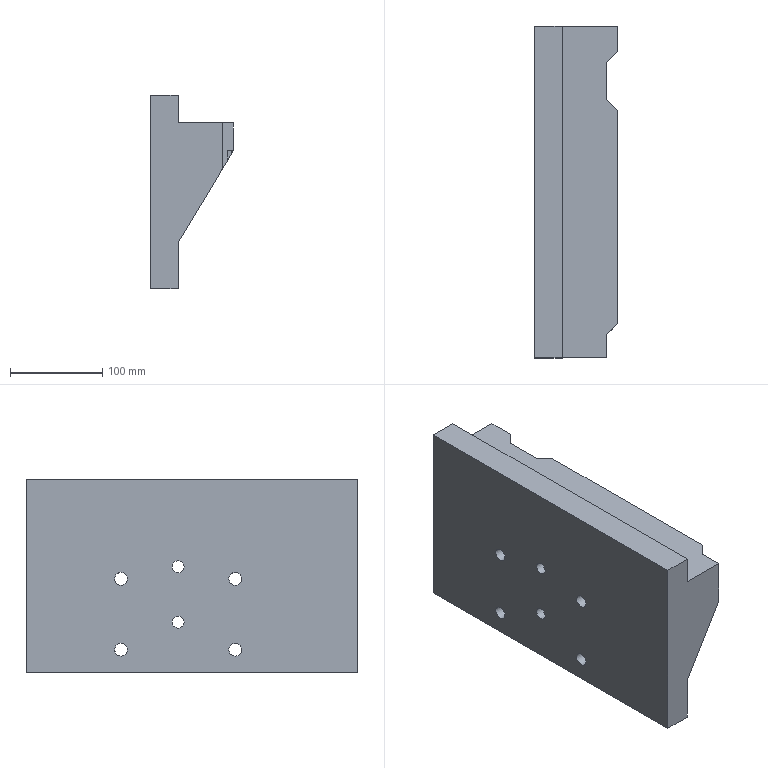Part | NX | features solid 2 | 1 solid | 34 faces | box 90 x 360 x 210 mm | volume 3029888 mm3 | plane 24 | cylinder 10 | commonest cylinder face diameters 14 x4 20 x4 13 x2
STEP:
#1=CARTESIAN_POINT('',(-737.,-445.,40.));
#2=VERTEX_POINT('',#1);
#3=CARTESIAN_POINT('',(-737.,-445.,-10.));
#4=VERTEX_POINT('',#3);
#5=CARTESIAN_POINT('',(-737.,-445.,14.964));
#6=DIRECTION('',(0.,0.,1.));
#7=VECTOR('',#6,1000.);
#8=LINE('',#5,#7);
#9=EDGE_CURVE('',#2,#4,#8,.F.);
#10=ORIENTED_EDGE('',*,*,#9,.F.);
#11=CARTESIAN_POINT('',(-785.,-445.,40.));
#12=VERTEX_POINT('',#11);
#13=CARTESIAN_POINT('',(-785.,-445.,40.));
#14=DIRECTION('',(1.,0.,0.));
#15=VECTOR('',#14,1000.);
#16=LINE('',#13,#15);
#17=EDGE_CURVE('',#12,#2,#16,.T.);
#18=ORIENTED_EDGE('',*,*,#17,.F.);
#19=CARTESIAN_POINT('',(-785.,-445.,70.));
#20=VERTEX_POINT('',#19);
#21=CARTESIAN_POINT('',(-785.,-445.,69.026));
#22=DIRECTION('',(0.,0.,1.));
#23=VECTOR('',#22,1000.);
#24=LINE('',#21,#23);
#25=EDGE_CURVE('',#20,#12,#24,.F.);
#26=ORIENTED_EDGE('',*,*,#25,.F.);
#27=CARTESIAN_POINT('',(-815.,-445.,70.));
#28=VERTEX_POINT('',#27);
#29=CARTESIAN_POINT('',(-785.,-445.,70.));
#30=DIRECTION('',(-1.,0.,0.));
#31=VECTOR('',#30,1000.);
#32=LINE('',#29,#31);
#33=EDGE_CURVE('',#20,#28,#32,.T.);
#34=ORIENTED_EDGE('',*,*,#33,.T.);
#35=CARTESIAN_POINT('',(-815.,-445.,-140.));
#36=VERTEX_POINT('',#35);
#37=CARTESIAN_POINT('',(-815.,-445.,69.026));
#38=DIRECTION('',(0.,0.,1.));
#39=VECTOR('',#38,1000.);
#40=LINE('',#37,#39);
#41=EDGE_CURVE('',#28,#36,#40,.F.);
#42=ORIENTED_EDGE('',*,*,#41,.T.);
#43=CARTESIAN_POINT('',(-785.,-445.,-140.));
#44=VERTEX_POINT('',#43);
#45=CARTESIAN_POINT('',(-815.,-445.,-140.));
#46=DIRECTION('',(-1.,0.,0.));
#47=VECTOR('',#46,1000.);
#48=LINE('',#45,#47);
#49=EDGE_CURVE('',#44,#36,#48,.T.);
#50=ORIENTED_EDGE('',*,*,#49,.F.);
#51=CARTESIAN_POINT('',(-785.,-445.,-90.));
#52=VERTEX_POINT('',#51);
#53=CARTESIAN_POINT('',(-785.,-445.,0.));
#54=DIRECTION('',(0.,0.,1.));
#55=VECTOR('',#54,1000.);
#56=LINE('',#53,#55);
#57=EDGE_CURVE('',#52,#44,#56,.F.);
#58=ORIENTED_EDGE('',*,*,#57,.F.);
#59=CARTESIAN_POINT('',(-740.882,-445.,-16.471));
#60=DIRECTION('',(-0.5145,0.,-0.8575));
#61=VECTOR('',#60,1000.);
#62=LINE('',#59,#61);
#63=EDGE_CURVE('',#4,#52,#62,.T.);
#64=ORIENTED_EDGE('',*,*,#63,.F.);
#65=EDGE_LOOP('',(#10,#18,#26,#34,#42,#50,#58,#64));
#66=FACE_BOUND('',#65,.T.);
#67=CARTESIAN_POINT('',(-785.,-445.,14.964));
#68=DIRECTION('',(0.,-1.,0.));
#69=DIRECTION('',(0.,0.,-1.));
#70=AXIS2_PLACEMENT_3D('',#67,#68,#69);
#71=PLANE('',#70);
#72=ADVANCED_FACE('',(#66),#71,.T.);
#73=CARTESIAN_POINT('',(-725.,-113.,40.));
#74=VERTEX_POINT('',#73);
#75=CARTESIAN_POINT('',(-725.,-85.,40.));
#76=VERTEX_POINT('',#75);
#77=CARTESIAN_POINT('',(-725.,-415.,40.));
#78=DIRECTION('',(0.,-1.,0.));
#79=VECTOR('',#78,1000.);
#80=LINE('',#77,#79);
#81=EDGE_CURVE('',#74,#76,#80,.F.);
#82=ORIENTED_EDGE('',*,*,#81,.F.);
#83=CARTESIAN_POINT('',(-725.,-113.,10.));
#84=VERTEX_POINT('',#83);
#85=CARTESIAN_POINT('',(-725.,-113.,60.));
#86=DIRECTION('',(0.,0.,-1.));
#87=VECTOR('',#86,1000.);
#88=LINE('',#85,#87);
#89=EDGE_CURVE('',#74,#84,#88,.T.);
#90=ORIENTED_EDGE('',*,*,#89,.T.);
#91=CARTESIAN_POINT('',(-725.,-85.,10.));
#92=VERTEX_POINT('',#91);
#93=CARTESIAN_POINT('',(-725.,-85.,10.));
#94=DIRECTION('',(0.,1.,0.));
#95=VECTOR('',#94,1000.);
#96=LINE('',#93,#95);
#97=EDGE_CURVE('',#84,#92,#96,.T.);
#98=ORIENTED_EDGE('',*,*,#97,.T.);
#99=CARTESIAN_POINT('',(-725.,-85.,69.026));
#100=DIRECTION('',(0.,0.,1.));
#101=VECTOR('',#100,1000.);
#102=LINE('',#99,#101);
#103=EDGE_CURVE('',#76,#92,#102,.F.);
#104=ORIENTED_EDGE('',*,*,#103,.F.);
#105=EDGE_LOOP('',(#82,#90,#98,#104));
#106=FACE_BOUND('',#105,.T.);
#107=CARTESIAN_POINT('',(-725.,-65.,29.026));
#108=DIRECTION('',(-1.,0.,0.));
#109=DIRECTION('',(0.,-1.,0.));
#110=AXIS2_PLACEMENT_3D('',#107,#108,#109);
#111=PLANE('',#110);
#112=ADVANCED_FACE('',(#106),#111,.F.);
#113=CARTESIAN_POINT('',(-815.,-195.,-115.));
#114=VERTEX_POINT('',#113);
#115=CARTESIAN_POINT('',(-815.,-188.,-115.));
#116=DIRECTION('',(-1.,0.,0.));
#117=DIRECTION('',(0.,-1.,0.));
#118=AXIS2_PLACEMENT_3D('',#115,#116,#117);
#119=CIRCLE('',#118,7.);
#120=EDGE_CURVE('',#114,#114,#119,.F.);
#121=ORIENTED_EDGE('',*,*,#120,.F.);
#122=EDGE_LOOP('',(#121));
#123=FACE_BOUND('',#122,.T.);
#124=CARTESIAN_POINT('',(-795.,-188.,-122.));
#125=VERTEX_POINT('',#124);
#126=CARTESIAN_POINT('',(-795.,-188.,-115.));
#127=DIRECTION('',(1.,0.,0.));
#128=DIRECTION('',(0.,0.,-1.));
#129=AXIS2_PLACEMENT_3D('',#126,#127,#128);
#130=CIRCLE('',#129,7.);
#131=EDGE_CURVE('',#125,#125,#130,.F.);
#132=ORIENTED_EDGE('',*,*,#131,.F.);
#133=EDGE_LOOP('',(#132));
#134=FACE_BOUND('',#133,.T.);
#135=CARTESIAN_POINT('',(-915.,-188.,-115.));
#136=DIRECTION('',(1.,0.,0.));
#137=DIRECTION('',(0.,0.,-1.));
#138=AXIS2_PLACEMENT_3D('',#135,#136,#137);
#139=CYLINDRICAL_SURFACE('',#138,7.);
#140=ADVANCED_FACE('',(#123,#134),#139,.F.);
#141=CARTESIAN_POINT('',(-785.,-198.,-115.));
#142=VERTEX_POINT('',#141);
#143=CARTESIAN_POINT('',(-785.,-188.,-115.));
#144=DIRECTION('',(-1.,0.,0.));
#145=DIRECTION('',(0.,-1.,0.));
#146=AXIS2_PLACEMENT_3D('',#143,#144,#145);
#147=CIRCLE('',#146,10.);
#148=EDGE_CURVE('',#142,#142,#147,.T.);
#149=ORIENTED_EDGE('',*,*,#148,.T.);
#150=EDGE_LOOP('',(#149));
#151=FACE_BOUND('',#150,.T.);
#152=CARTESIAN_POINT('',(-785.,-322.,-115.));
#153=VERTEX_POINT('',#152);
#154=CARTESIAN_POINT('',(-785.,-312.,-115.));
#155=DIRECTION('',(-1.,0.,0.));
#156=DIRECTION('',(0.,-1.,0.));
#157=AXIS2_PLACEMENT_3D('',#154,#155,#156);
#158=CIRCLE('',#157,10.);
#159=EDGE_CURVE('',#153,#153,#158,.T.);
#160=ORIENTED_EDGE('',*,*,#159,.T.);
#161=EDGE_LOOP('',(#160));
#162=FACE_BOUND('',#161,.T.);
#163=CARTESIAN_POINT('',(-785.,-198.,-38.));
#164=VERTEX_POINT('',#163);
#165=CARTESIAN_POINT('',(-785.,-188.,-38.));
#166=DIRECTION('',(-1.,0.,0.));
#167=DIRECTION('',(0.,-1.,0.));
#168=AXIS2_PLACEMENT_3D('',#165,#166,#167);
#169=CIRCLE('',#168,10.);
#170=EDGE_CURVE('',#164,#164,#169,.T.);
#171=ORIENTED_EDGE('',*,*,#170,.T.);
#172=EDGE_LOOP('',(#171));
#173=FACE_BOUND('',#172,.T.);
#174=CARTESIAN_POINT('',(-785.,-322.,-38.));
#175=VERTEX_POINT('',#174);
#176=CARTESIAN_POINT('',(-785.,-312.,-38.));
#177=DIRECTION('',(-1.,0.,0.));
#178=DIRECTION('',(0.,-1.,0.));
#179=AXIS2_PLACEMENT_3D('',#176,#177,#178);
#180=CIRCLE('',#179,10.);
#181=EDGE_CURVE('',#175,#175,#180,.T.);
#182=ORIENTED_EDGE('',*,*,#181,.T.);
#183=EDGE_LOOP('',(#182));
#184=FACE_BOUND('',#183,.T.);
#185=CARTESIAN_POINT('',(-785.,-256.5,-25.));
#186=VERTEX_POINT('',#185);
#187=CARTESIAN_POINT('',(-785.,-250.,-25.));
#188=DIRECTION('',(-1.,0.,0.));
#189=DIRECTION('',(0.,-1.,0.));
#190=AXIS2_PLACEMENT_3D('',#187,#188,#189);
#191=CIRCLE('',#190,6.5);
#192=EDGE_CURVE('',#186,#186,#191,.T.);
#193=ORIENTED_EDGE('',*,*,#192,.T.);
#194=EDGE_LOOP('',(#193));
#195=FACE_BOUND('',#194,.T.);
#196=CARTESIAN_POINT('',(-785.,-256.5,-85.));
#197=VERTEX_POINT('',#196);
#198=CARTESIAN_POINT('',(-785.,-250.,-85.));
#199=DIRECTION('',(-1.,0.,0.));
#200=DIRECTION('',(0.,-1.,0.));
#201=AXIS2_PLACEMENT_3D('',#198,#199,#200);
#202=CIRCLE('',#201,6.5);
#203=EDGE_CURVE('',#197,#197,#202,.T.);
#204=ORIENTED_EDGE('',*,*,#203,.T.);
#205=EDGE_LOOP('',(#204));
#206=FACE_BOUND('',#205,.T.);
#207=CARTESIAN_POINT('',(-785.,-415.,10.));
#208=VERTEX_POINT('',#207);
#209=CARTESIAN_POINT('',(-785.,-415.,-90.));
#210=VERTEX_POINT('',#209);
#211=CARTESIAN_POINT('',(-785.,-415.,10.));
#212=DIRECTION('',(0.,0.,-1.));
#213=VECTOR('',#212,1000.);
#214=LINE('',#211,#213);
#215=EDGE_CURVE('',#208,#210,#214,.T.);
#216=ORIENTED_EDGE('',*,*,#215,.T.);
#217=CARTESIAN_POINT('',(-785.,-445.,-90.));
#218=DIRECTION('',(0.,1.,0.));
#219=VECTOR('',#218,1000.);
#220=LINE('',#217,#219);
#221=EDGE_CURVE('',#52,#210,#220,.T.);
#222=ORIENTED_EDGE('',*,*,#221,.F.);
#223=ORIENTED_EDGE('',*,*,#57,.T.);
#224=CARTESIAN_POINT('',(-785.,-85.,-140.));
#225=VERTEX_POINT('',#224);
#226=CARTESIAN_POINT('',(-785.,-65.,-140.));
#227=DIRECTION('',(0.,-1.,0.));
#228=VECTOR('',#227,1000.);
#229=LINE('',#226,#228);
#230=EDGE_CURVE('',#44,#225,#229,.F.);
#231=ORIENTED_EDGE('',*,*,#230,.T.);
#232=CARTESIAN_POINT('',(-785.,-85.,-90.));
#233=VERTEX_POINT('',#232);
#234=CARTESIAN_POINT('',(-785.,-85.,69.026));
#235=DIRECTION('',(0.,0.,-1.));
#236=VECTOR('',#235,1000.);
#237=LINE('',#234,#236);
#238=EDGE_CURVE('',#233,#225,#237,.T.);
#239=ORIENTED_EDGE('',*,*,#238,.F.);
#240=CARTESIAN_POINT('',(-785.,-115.,-90.));
#241=VERTEX_POINT('',#240);
#242=CARTESIAN_POINT('',(-785.,-85.,-90.));
#243=DIRECTION('',(0.,1.,0.));
#244=VECTOR('',#243,1000.);
#245=LINE('',#242,#244);
#246=EDGE_CURVE('',#241,#233,#245,.T.);
#247=ORIENTED_EDGE('',*,*,#246,.F.);
#248=CARTESIAN_POINT('',(-785.,-115.,10.));
#249=VERTEX_POINT('',#248);
#250=CARTESIAN_POINT('',(-785.,-115.,10.));
#251=DIRECTION('',(0.,0.,1.));
#252=VECTOR('',#251,1000.);
#253=LINE('',#250,#252);
#254=EDGE_CURVE('',#249,#241,#253,.F.);
#255=ORIENTED_EDGE('',*,*,#254,.F.);
#256=CARTESIAN_POINT('',(-785.,-65.,10.));
#257=DIRECTION('',(0.,1.,0.));
#258=VECTOR('',#257,1000.);
#259=LINE('',#256,#258);
#260=EDGE_CURVE('',#208,#249,#259,.T.);
#261=ORIENTED_EDGE('',*,*,#260,.F.);
#262=EDGE_LOOP('',(#216,#222,#223,#231,#239,#247,#255,#261));
#263=FACE_BOUND('',#262,.T.);
#264=CARTESIAN_POINT('',(-785.,-65.,69.026));
#265=DIRECTION('',(-1.,0.,0.));
#266=DIRECTION('',(0.,-1.,0.));
#267=AXIS2_PLACEMENT_3D('',#264,#265,#266);
#268=PLANE('',#267);
#269=ADVANCED_FACE('',(#151,#162,#173,#184,#195,#206,#263),#268,.F.);
#270=CARTESIAN_POINT('',(-725.,-408.,10.));
#271=VERTEX_POINT('',#270);
#272=CARTESIAN_POINT('',(-725.,-177.,10.));
#273=VERTEX_POINT('',#272);
#274=CARTESIAN_POINT('',(-725.,-65.,10.));
#275=DIRECTION('',(0.,1.,0.));
#276=VECTOR('',#275,1000.);
#277=LINE('',#274,#276);
#278=EDGE_CURVE('',#271,#273,#277,.T.);
#279=ORIENTED_EDGE('',*,*,#278,.F.);
#280=CARTESIAN_POINT('',(-732.,-415.,10.));
#281=VERTEX_POINT('',#280);
#282=CARTESIAN_POINT('',(-758.5,-441.5,10.));
#283=DIRECTION('',(-0.7071,-0.7071,0.));
#284=VECTOR('',#283,1000.);
#285=LINE('',#282,#284);
#286=EDGE_CURVE('',#271,#281,#285,.T.);
#287=ORIENTED_EDGE('',*,*,#286,.T.);
#288=CARTESIAN_POINT('',(-785.,-415.,10.));
#289=DIRECTION('',(1.,0.,0.));
#290=VECTOR('',#289,1000.);
#291=LINE('',#288,#290);
#292=EDGE_CURVE('',#208,#281,#291,.T.);
#293=ORIENTED_EDGE('',*,*,#292,.F.);
#294=ORIENTED_EDGE('',*,*,#260,.T.);
#295=CARTESIAN_POINT('',(-727.,-115.,10.));
#296=VERTEX_POINT('',#295);
#297=CARTESIAN_POINT('',(-785.,-115.,10.));
#298=DIRECTION('',(1.,0.,0.));
#299=VECTOR('',#298,1000.);
#300=LINE('',#297,#299);
#301=EDGE_CURVE('',#249,#296,#300,.T.);
#302=ORIENTED_EDGE('',*,*,#301,.T.);
#303=CARTESIAN_POINT('',(-737.,-125.,10.));
#304=VERTEX_POINT('',#303);
#305=CARTESIAN_POINT('',(-906.,-294.,10.));
#306=DIRECTION('',(-0.7071,-0.7071,0.));
#307=VECTOR('',#306,1000.);
#308=LINE('',#305,#307);
#309=EDGE_CURVE('',#296,#304,#308,.T.);
#310=ORIENTED_EDGE('',*,*,#309,.T.);
#311=CARTESIAN_POINT('',(-737.,-165.,10.));
#312=VERTEX_POINT('',#311);
#313=CARTESIAN_POINT('',(-737.,-415.,10.));
#314=DIRECTION('',(0.,1.,0.));
#315=VECTOR('',#314,1000.);
#316=LINE('',#313,#315);
#317=EDGE_CURVE('',#312,#304,#316,.T.);
#318=ORIENTED_EDGE('',*,*,#317,.F.);
#319=CARTESIAN_POINT('',(-636.,-266.,10.));
#320=DIRECTION('',(0.7071,-0.7071,0.));
#321=VECTOR('',#320,1000.);
#322=LINE('',#319,#321);
#323=EDGE_CURVE('',#312,#273,#322,.T.);
#324=ORIENTED_EDGE('',*,*,#323,.T.);
#325=EDGE_LOOP('',(#279,#287,#293,#294,#302,#310,#318,#324));
#326=FACE_BOUND('',#325,.T.);
#327=CARTESIAN_POINT('',(-785.,-415.,10.));
#328=DIRECTION('',(0.,0.,1.));
#329=DIRECTION('',(0.,1.,0.));
#330=AXIS2_PLACEMENT_3D('',#327,#328,#329);
#331=PLANE('',#330);
#332=ADVANCED_FACE('',(#326),#331,.F.);
#333=CARTESIAN_POINT('',(-815.,-319.,-38.));
#334=VERTEX_POINT('',#333);
#335=CARTESIAN_POINT('',(-815.,-312.,-38.));
#336=DIRECTION('',(-1.,0.,0.));
#337=DIRECTION('',(0.,-1.,0.));
#338=AXIS2_PLACEMENT_3D('',#335,#336,#337);
#339=CIRCLE('',#338,7.);
#340=EDGE_CURVE('',#334,#334,#339,.F.);
#341=ORIENTED_EDGE('',*,*,#340,.T.);
#342=EDGE_LOOP('',(#341));
#343=FACE_BOUND('',#342,.T.);
#344=CARTESIAN_POINT('',(-815.,-319.,-115.));
#345=VERTEX_POINT('',#344);
#346=CARTESIAN_POINT('',(-815.,-312.,-115.));
#347=DIRECTION('',(-1.,0.,0.));
#348=DIRECTION('',(0.,-1.,0.));
#349=AXIS2_PLACEMENT_3D('',#346,#347,#348);
#350=CIRCLE('',#349,7.);
#351=EDGE_CURVE('',#345,#345,#350,.F.);
#352=ORIENTED_EDGE('',*,*,#351,.T.);
#353=EDGE_LOOP('',(#352));
#354=FACE_BOUND('',#353,.T.);
#355=CARTESIAN_POINT('',(-815.,-85.,-140.));
#356=VERTEX_POINT('',#355);
#357=CARTESIAN_POINT('',(-815.,-65.,-140.));
#358=DIRECTION('',(0.,-1.,0.));
#359=VECTOR('',#358,1000.);
#360=LINE('',#357,#359);
#361=EDGE_CURVE('',#36,#356,#360,.F.);
#362=ORIENTED_EDGE('',*,*,#361,.F.);
#363=ORIENTED_EDGE('',*,*,#41,.F.);
#364=CARTESIAN_POINT('',(-815.,-85.,70.));
#365=VERTEX_POINT('',#364);
#366=CARTESIAN_POINT('',(-815.,-250.,70.));
#367=DIRECTION('',(0.,-1.,0.));
#368=VECTOR('',#367,1000.);
#369=LINE('',#366,#368);
#370=EDGE_CURVE('',#28,#365,#369,.F.);
#371=ORIENTED_EDGE('',*,*,#370,.T.);
#372=CARTESIAN_POINT('',(-815.,-85.,69.026));
#373=DIRECTION('',(0.,0.,1.));
#374=VECTOR('',#373,1000.);
#375=LINE('',#372,#374);
#376=EDGE_CURVE('',#365,#356,#375,.F.);
#377=ORIENTED_EDGE('',*,*,#376,.T.);
#378=EDGE_LOOP('',(#362,#363,#371,#377));
#379=FACE_BOUND('',#378,.T.);
#380=CARTESIAN_POINT('',(-815.,-256.5,-85.));
#381=VERTEX_POINT('',#380);
#382=CARTESIAN_POINT('',(-815.,-250.,-85.));
#383=DIRECTION('',(-1.,0.,0.));
#384=DIRECTION('',(0.,-1.,0.));
#385=AXIS2_PLACEMENT_3D('',#382,#383,#384);
#386=CIRCLE('',#385,6.5);
#387=EDGE_CURVE('',#381,#381,#386,.T.);
#388=ORIENTED_EDGE('',*,*,#387,.F.);
#389=EDGE_LOOP('',(#388));
#390=FACE_BOUND('',#389,.T.);
#391=ORIENTED_EDGE('',*,*,#120,.T.);
#392=EDGE_LOOP('',(#391));
#393=FACE_BOUND('',#392,.T.);
#394=CARTESIAN_POINT('',(-815.,-256.5,-25.));
#395=VERTEX_POINT('',#394);
#396=CARTESIAN_POINT('',(-815.,-250.,-25.));
#397=DIRECTION('',(-1.,0.,0.));
#398=DIRECTION('',(0.,-1.,0.));
#399=AXIS2_PLACEMENT_3D('',#396,#397,#398);
#400=CIRCLE('',#399,6.5);
#401=EDGE_CURVE('',#395,#395,#400,.T.);
#402=ORIENTED_EDGE('',*,*,#401,.F.);
#403=EDGE_LOOP('',(#402));
#404=FACE_BOUND('',#403,.T.);
#405=CARTESIAN_POINT('',(-815.,-195.,-38.));
#406=VERTEX_POINT('',#405);
#407=CARTESIAN_POINT('',(-815.,-188.,-38.));
#408=DIRECTION('',(-1.,0.,0.));
#409=DIRECTION('',(0.,-1.,0.));
#410=AXIS2_PLACEMENT_3D('',#407,#408,#409);
#411=CIRCLE('',#410,7.);
#412=EDGE_CURVE('',#406,#406,#411,.F.);
#413=ORIENTED_EDGE('',*,*,#412,.T.);
#414=EDGE_LOOP('',(#413));
#415=FACE_BOUND('',#414,.T.);
#416=CARTESIAN_POINT('',(-815.,-65.,69.026));
#417=DIRECTION('',(-1.,0.,0.));
#418=DIRECTION('',(0.,-1.,0.));
#419=AXIS2_PLACEMENT_3D('',#416,#417,#418);
#420=PLANE('',#419);
#421=ADVANCED_FACE('',(#343,#354,#379,#390,#393,#404,#415),#420,.T.);
#422=CARTESIAN_POINT('',(-785.,-85.,40.));
#423=VERTEX_POINT('',#422);
#424=CARTESIAN_POINT('',(-785.,-415.,40.));
#425=DIRECTION('',(0.,-1.,0.));
#426=VECTOR('',#425,1000.);
#427=LINE('',#424,#426);
#428=EDGE_CURVE('',#12,#423,#427,.F.);
#429=ORIENTED_EDGE('',*,*,#428,.T.);
#430=CARTESIAN_POINT('',(-785.,-85.,70.));
#431=VERTEX_POINT('',#430);
#432=CARTESIAN_POINT('',(-785.,-85.,69.026));
#433=DIRECTION('',(0.,0.,1.));
#434=VECTOR('',#433,1000.);
#435=LINE('',#432,#434);
#436=EDGE_CURVE('',#431,#423,#435,.F.);
#437=ORIENTED_EDGE('',*,*,#436,.F.);
#438=CARTESIAN_POINT('',(-785.,-250.,70.));
#439=DIRECTION('',(0.,-1.,0.));
#440=VECTOR('',#439,1000.);
#441=LINE('',#438,#440);
#442=EDGE_CURVE('',#20,#431,#441,.F.);
#443=ORIENTED_EDGE('',*,*,#442,.F.);
#444=ORIENTED_EDGE('',*,*,#25,.T.);
#445=EDGE_LOOP('',(#429,#437,#443,#444));
#446=FACE_BOUND('',#445,.T.);
#447=CARTESIAN_POINT('',(-785.,-65.,69.026));
#448=DIRECTION('',(-1.,0.,0.));
#449=DIRECTION('',(0.,-1.,0.));
#450=AXIS2_PLACEMENT_3D('',#447,#448,#449);
#451=PLANE('',#450);
#452=ADVANCED_FACE('',(#446),#451,.F.);
#453=CARTESIAN_POINT('',(-785.,-85.,70.));
#454=DIRECTION('',(-1.,0.,0.));
#455=VECTOR('',#454,1000.);
#456=LINE('',#453,#455);
#457=EDGE_CURVE('',#431,#365,#456,.T.);
#458=ORIENTED_EDGE('',*,*,#457,.T.);
#459=ORIENTED_EDGE('',*,*,#370,.F.);
#460=ORIENTED_EDGE('',*,*,#33,.F.);
#461=ORIENTED_EDGE('',*,*,#442,.T.);
#462=EDGE_LOOP('',(#458,#459,#460,#461));
#463=FACE_BOUND('',#462,.T.);
#464=CARTESIAN_POINT('',(-890.,-250.,70.));
#465=DIRECTION('',(0.,0.,1.));
#466=DIRECTION('',(1.,0.,0.));
#467=AXIS2_PLACEMENT_3D('',#464,#465,#466);
#468=PLANE('',#467);
#469=ADVANCED_FACE('',(#463),#468,.T.);
#470=CARTESIAN_POINT('',(-815.,-85.,-140.));
#471=DIRECTION('',(-1.,0.,0.));
#472=VECTOR('',#471,1000.);
#473=LINE('',#470,#472);
#474=EDGE_CURVE('',#225,#356,#473,.T.);
#475=ORIENTED_EDGE('',*,*,#474,.F.);
#476=ORIENTED_EDGE('',*,*,#230,.F.);
#477=ORIENTED_EDGE('',*,*,#49,.T.);
#478=ORIENTED_EDGE('',*,*,#361,.T.);
#479=EDGE_LOOP('',(#475,#476,#477,#478));
#480=FACE_BOUND('',#479,.T.);
#481=CARTESIAN_POINT('',(-815.,-250.,-140.));
#482=DIRECTION('',(0.,0.,-1.));
#483=DIRECTION('',(-1.,0.,0.));
#484=AXIS2_PLACEMENT_3D('',#481,#482,#483);
#485=PLANE('',#484);
#486=ADVANCED_FACE('',(#480),#485,.T.);
#487=CARTESIAN_POINT('',(-714.841,-85.,26.931));
#488=DIRECTION('',(0.5145,0.,0.8575));
#489=VECTOR('',#488,1000.);
#490=LINE('',#487,#489);
#491=EDGE_CURVE('',#92,#233,#490,.F.);
#492=ORIENTED_EDGE('',*,*,#491,.T.);
#493=ORIENTED_EDGE('',*,*,#238,.T.);
#494=ORIENTED_EDGE('',*,*,#474,.T.);
#495=ORIENTED_EDGE('',*,*,#376,.F.);
#496=ORIENTED_EDGE('',*,*,#457,.F.);
#497=ORIENTED_EDGE('',*,*,#436,.T.);
#498=CARTESIAN_POINT('',(-785.,-85.,40.));
#499=DIRECTION('',(1.,0.,0.));
#500=VECTOR('',#499,1000.);
#501=LINE('',#498,#500);
#502=EDGE_CURVE('',#423,#76,#501,.T.);
#503=ORIENTED_EDGE('',*,*,#502,.T.);
#504=ORIENTED_EDGE('',*,*,#103,.T.);
#505=EDGE_LOOP('',(#492,#493,#494,#495,#496,#497,#503,#504));
#506=FACE_BOUND('',#505,.T.);
#507=CARTESIAN_POINT('',(-785.,-85.,69.026));
#508=DIRECTION('',(0.,1.,0.));
#509=DIRECTION('',(0.,0.,-1.));
#510=AXIS2_PLACEMENT_3D('',#507,#508,#509);
#511=PLANE('',#510);
#512=ADVANCED_FACE('',(#506),#511,.T.);
#513=CARTESIAN_POINT('',(-725.,-408.,40.));
#514=VERTEX_POINT('',#513);
#515=CARTESIAN_POINT('',(-725.,-177.,40.));
#516=VERTEX_POINT('',#515);
#517=CARTESIAN_POINT('',(-725.,-415.,40.));
#518=DIRECTION('',(0.,-1.,0.));
#519=VECTOR('',#518,1000.);
#520=LINE('',#517,#519);
#521=EDGE_CURVE('',#514,#516,#520,.F.);
#522=ORIENTED_EDGE('',*,*,#521,.F.);
#523=CARTESIAN_POINT('',(-725.,-408.,60.));
#524=DIRECTION('',(0.,0.,-1.));
#525=VECTOR('',#524,1000.);
#526=LINE('',#523,#525);
#527=EDGE_CURVE('',#514,#271,#526,.T.);
#528=ORIENTED_EDGE('',*,*,#527,.T.);
#529=ORIENTED_EDGE('',*,*,#278,.T.);
#530=CARTESIAN_POINT('',(-725.,-177.,60.));
#531=DIRECTION('',(0.,0.,-1.));
#532=VECTOR('',#531,1000.);
#533=LINE('',#530,#532);
#534=EDGE_CURVE('',#516,#273,#533,.T.);
#535=ORIENTED_EDGE('',*,*,#534,.F.);
#536=EDGE_LOOP('',(#522,#528,#529,#535));
#537=FACE_BOUND('',#536,.T.);
#538=CARTESIAN_POINT('',(-725.,-65.,29.026));
#539=DIRECTION('',(-1.,0.,0.));
#540=DIRECTION('',(0.,-1.,0.));
#541=AXIS2_PLACEMENT_3D('',#538,#539,#540);
#542=PLANE('',#541);
#543=ADVANCED_FACE('',(#537),#542,.F.);
#544=CARTESIAN_POINT('',(-737.,-420.,40.));
#545=VERTEX_POINT('',#544);
#546=CARTESIAN_POINT('',(-737.,-415.,40.));
#547=DIRECTION('',(0.,1.,0.));
#548=VECTOR('',#547,1000.);
#549=LINE('',#546,#548);
#550=EDGE_CURVE('',#545,#2,#549,.F.);
#551=ORIENTED_EDGE('',*,*,#550,.F.);
#552=CARTESIAN_POINT('',(-758.5,-441.5,40.));
#553=DIRECTION('',(-0.7071,-0.7071,0.));
#554=VECTOR('',#553,1000.);
#555=LINE('',#552,#554);
#556=EDGE_CURVE('',#545,#514,#555,.F.);
#557=ORIENTED_EDGE('',*,*,#556,.T.);
#558=ORIENTED_EDGE('',*,*,#521,.T.);
#559=CARTESIAN_POINT('',(-737.,-165.,40.));
#560=VERTEX_POINT('',#559);
#561=CARTESIAN_POINT('',(-636.,-266.,40.));
#562=DIRECTION('',(0.7071,-0.7071,0.));
#563=VECTOR('',#562,1000.);
#564=LINE('',#561,#563);
#565=EDGE_CURVE('',#516,#560,#564,.F.);
#566=ORIENTED_EDGE('',*,*,#565,.T.);
#567=CARTESIAN_POINT('',(-737.,-125.,40.));
#568=VERTEX_POINT('',#567);
#569=CARTESIAN_POINT('',(-737.,-415.,40.));
#570=DIRECTION('',(0.,1.,0.));
#571=VECTOR('',#570,1000.);
#572=LINE('',#569,#571);
#573=EDGE_CURVE('',#568,#560,#572,.F.);
#574=ORIENTED_EDGE('',*,*,#573,.F.);
#575=CARTESIAN_POINT('',(-906.,-294.,40.));
#576=DIRECTION('',(-0.7071,-0.7071,0.));
#577=VECTOR('',#576,1000.);
#578=LINE('',#575,#577);
#579=EDGE_CURVE('',#568,#74,#578,.F.);
#580=ORIENTED_EDGE('',*,*,#579,.T.);
#581=ORIENTED_EDGE('',*,*,#81,.T.);
#582=ORIENTED_EDGE('',*,*,#502,.F.);
#583=ORIENTED_EDGE('',*,*,#428,.F.);
#584=ORIENTED_EDGE('',*,*,#17,.T.);
#585=EDGE_LOOP('',(#551,#557,#558,#566,#574,#580,#581,#582,#583,#584));
#586=FACE_BOUND('',#585,.T.);
#587=CARTESIAN_POINT('',(-785.,-415.,40.));
#588=DIRECTION('',(0.,0.,1.));
#589=DIRECTION('',(0.,1.,0.));
#590=AXIS2_PLACEMENT_3D('',#587,#588,#589);
#591=PLANE('',#590);
#592=ADVANCED_FACE('',(#586),#591,.T.);
#593=CARTESIAN_POINT('',(-795.,-312.,-122.));
#594=VERTEX_POINT('',#593);
#595=CARTESIAN_POINT('',(-795.,-312.,-115.));
#596=DIRECTION('',(1.,0.,0.));
#597=DIRECTION('',(0.,0.,-1.));
#598=AXIS2_PLACEMENT_3D('',#595,#596,#597);
#599=CIRCLE('',#598,7.);
#600=EDGE_CURVE('',#594,#594,#599,.F.);
#601=ORIENTED_EDGE('',*,*,#600,.F.);
#602=EDGE_LOOP('',(#601));
#603=FACE_BOUND('',#602,.T.);
#604=ORIENTED_EDGE('',*,*,#351,.F.);
#605=EDGE_LOOP('',(#604));
#606=FACE_BOUND('',#605,.T.);
#607=CARTESIAN_POINT('',(-915.,-312.,-115.));
#608=DIRECTION('',(1.,0.,0.));
#609=DIRECTION('',(0.,0.,-1.));
#610=AXIS2_PLACEMENT_3D('',#607,#608,#609);
#611=CYLINDRICAL_SURFACE('',#610,7.);
#612=ADVANCED_FACE('',(#603,#606),#611,.F.);
#613=ORIENTED_EDGE('',*,*,#387,.T.);
#614=EDGE_LOOP('',(#613));
#615=FACE_BOUND('',#614,.T.);
#616=ORIENTED_EDGE('',*,*,#203,.F.);
#617=EDGE_LOOP('',(#616));
#618=FACE_BOUND('',#617,.T.);
#619=CARTESIAN_POINT('',(-915.,-250.,-85.));
#620=DIRECTION('',(1.,0.,0.));
#621=DIRECTION('',(0.,0.,-1.));
#622=AXIS2_PLACEMENT_3D('',#619,#620,#621);
#623=CYLINDRICAL_SURFACE('',#622,6.5);
#624=ADVANCED_FACE('',(#615,#618),#623,.F.);
#625=CARTESIAN_POINT('',(-795.,-312.,-45.));
#626=VERTEX_POINT('',#625);
#627=CARTESIAN_POINT('',(-795.,-312.,-38.));
#628=DIRECTION('',(1.,0.,0.));
#629=DIRECTION('',(0.,0.,-1.));
#630=AXIS2_PLACEMENT_3D('',#627,#628,#629);
#631=CIRCLE('',#630,7.);
#632=EDGE_CURVE('',#626,#626,#631,.F.);
#633=ORIENTED_EDGE('',*,*,#632,.F.);
#634=EDGE_LOOP('',(#633));
#635=FACE_BOUND('',#634,.T.);
#636=ORIENTED_EDGE('',*,*,#340,.F.);
#637=EDGE_LOOP('',(#636));
#638=FACE_BOUND('',#637,.T.);
#639=CARTESIAN_POINT('',(-915.,-312.,-38.));
#640=DIRECTION('',(1.,0.,0.));
#641=DIRECTION('',(0.,0.,-1.));
#642=AXIS2_PLACEMENT_3D('',#639,#640,#641);
#643=CYLINDRICAL_SURFACE('',#642,7.);
#644=ADVANCED_FACE('',(#635,#638),#643,.F.);
#645=ORIENTED_EDGE('',*,*,#401,.T.);
#646=EDGE_LOOP('',(#645));
#647=FACE_BOUND('',#646,.T.);
#648=ORIENTED_EDGE('',*,*,#192,.F.);
#649=EDGE_LOOP('',(#648));
#650=FACE_BOUND('',#649,.T.);
#651=CARTESIAN_POINT('',(-915.,-250.,-25.));
#652=DIRECTION('',(1.,0.,0.));
#653=DIRECTION('',(0.,0.,-1.));
#654=AXIS2_PLACEMENT_3D('',#651,#652,#653);
#655=CYLINDRICAL_SURFACE('',#654,6.5);
#656=ADVANCED_FACE('',(#647,#650),#655,.F.);
#657=CARTESIAN_POINT('',(-795.,-188.,-45.));
#658=VERTEX_POINT('',#657);
#659=CARTESIAN_POINT('',(-795.,-188.,-38.));
#660=DIRECTION('',(1.,0.,0.));
#661=DIRECTION('',(0.,0.,-1.));
#662=AXIS2_PLACEMENT_3D('',#659,#660,#661);
#663=CIRCLE('',#662,7.);
#664=EDGE_CURVE('',#658,#658,#663,.F.);
#665=ORIENTED_EDGE('',*,*,#664,.F.);
#666=EDGE_LOOP('',(#665));
#667=FACE_BOUND('',#666,.T.);
#668=ORIENTED_EDGE('',*,*,#412,.F.);
#669=EDGE_LOOP('',(#668));
#670=FACE_BOUND('',#669,.T.);
#671=CARTESIAN_POINT('',(-915.,-188.,-38.));
#672=DIRECTION('',(1.,0.,0.));
#673=DIRECTION('',(0.,0.,-1.));
#674=AXIS2_PLACEMENT_3D('',#671,#672,#673);
#675=CYLINDRICAL_SURFACE('',#674,7.);
#676=ADVANCED_FACE('',(#667,#670),#675,.F.);
#677=CARTESIAN_POINT('',(-727.,-115.,6.667));
#678=VERTEX_POINT('',#677);
#679=CARTESIAN_POINT('',(-727.,-115.,10.));
#680=DIRECTION('',(0.,0.,-1.));
#681=VECTOR('',#680,1000.);
#682=LINE('',#679,#681);
#683=EDGE_CURVE('',#296,#678,#682,.T.);
#684=ORIENTED_EDGE('',*,*,#683,.F.);
#685=ORIENTED_EDGE('',*,*,#301,.F.);
#686=ORIENTED_EDGE('',*,*,#254,.T.);
#687=CARTESIAN_POINT('',(-740.882,-115.,-16.471));
#688=DIRECTION('',(-0.5145,0.,-0.8575));
#689=VECTOR('',#688,1000.);
#690=LINE('',#687,#689);
#691=EDGE_CURVE('',#678,#241,#690,.T.);
#692=ORIENTED_EDGE('',*,*,#691,.F.);
#693=EDGE_LOOP('',(#684,#685,#686,#692));
#694=FACE_BOUND('',#693,.T.);
#695=CARTESIAN_POINT('',(-785.,-115.,10.));
#696=DIRECTION('',(0.,-1.,0.));
#697=DIRECTION('',(0.,0.,-1.));
#698=AXIS2_PLACEMENT_3D('',#695,#696,#697);
#699=PLANE('',#698);
#700=ADVANCED_FACE('',(#694),#699,.T.);
#701=ORIENTED_EDGE('',*,*,#97,.F.);
#702=CARTESIAN_POINT('',(-766.581,-154.581,-59.302));
#703=DIRECTION('',(-0.4575,-0.4575,-0.7625));
#704=VECTOR('',#703,1000.);
#705=LINE('',#702,#704);
#706=EDGE_CURVE('',#84,#678,#705,.T.);
#707=ORIENTED_EDGE('',*,*,#706,.T.);
#708=ORIENTED_EDGE('',*,*,#691,.T.);
#709=ORIENTED_EDGE('',*,*,#246,.T.);
#710=ORIENTED_EDGE('',*,*,#491,.F.);
#711=EDGE_LOOP('',(#701,#707,#708,#709,#710));
#712=FACE_BOUND('',#711,.T.);
#713=CARTESIAN_POINT('',(-785.,-85.,-90.));
#714=DIRECTION('',(-0.8575,0.,0.5145));
#715=DIRECTION('',(0.5145,0.,0.8575));
#716=AXIS2_PLACEMENT_3D('',#713,#714,#715);
#717=PLANE('',#716);
#718=ADVANCED_FACE('',(#712),#717,.F.);
#719=ORIENTED_EDGE('',*,*,#292,.T.);
#720=CARTESIAN_POINT('',(-732.,-415.,-1.667));
#721=VERTEX_POINT('',#720);
#722=CARTESIAN_POINT('',(-732.,-415.,10.));
#723=DIRECTION('',(0.,0.,-1.));
#724=VECTOR('',#723,1000.);
#725=LINE('',#722,#724);
#726=EDGE_CURVE('',#281,#721,#725,.T.);
#727=ORIENTED_EDGE('',*,*,#726,.T.);
#728=CARTESIAN_POINT('',(-740.882,-415.,-16.471));
#729=DIRECTION('',(-0.5145,0.,-0.8575));
#730=VECTOR('',#729,1000.);
#731=LINE('',#728,#730);
#732=EDGE_CURVE('',#721,#210,#731,.T.);
#733=ORIENTED_EDGE('',*,*,#732,.T.);
#734=ORIENTED_EDGE('',*,*,#215,.F.);
#735=EDGE_LOOP('',(#719,#727,#733,#734));
#736=FACE_BOUND('',#735,.T.);
#737=CARTESIAN_POINT('',(-785.,-415.,10.));
#738=DIRECTION('',(0.,-1.,0.));
#739=DIRECTION('',(0.,0.,-1.));
#740=AXIS2_PLACEMENT_3D('',#737,#738,#739);
#741=PLANE('',#740);
#742=ADVANCED_FACE('',(#736),#741,.F.);
#743=ORIENTED_EDGE('',*,*,#732,.F.);
#744=CARTESIAN_POINT('',(-737.,-420.,-10.));
#745=VERTEX_POINT('',#744);
#746=CARTESIAN_POINT('',(-773.907,-456.907,-71.512));
#747=DIRECTION('',(-0.4575,-0.4575,-0.7625));
#748=VECTOR('',#747,1000.);
#749=LINE('',#746,#748);
#750=EDGE_CURVE('',#721,#745,#749,.T.);
#751=ORIENTED_EDGE('',*,*,#750,.T.);
#752=CARTESIAN_POINT('',(-737.,-415.,-10.));
#753=DIRECTION('',(0.,1.,0.));
#754=VECTOR('',#753,1000.);
#755=LINE('',#752,#754);
#756=EDGE_CURVE('',#4,#745,#755,.T.);
#757=ORIENTED_EDGE('',*,*,#756,.F.);
#758=ORIENTED_EDGE('',*,*,#63,.T.);
#759=ORIENTED_EDGE('',*,*,#221,.T.);
#760=EDGE_LOOP('',(#743,#751,#757,#758,#759));
#761=FACE_BOUND('',#760,.T.);
#762=CARTESIAN_POINT('',(-785.,-415.,-90.));
#763=DIRECTION('',(-0.8575,0.,0.5145));
#764=DIRECTION('',(0.5145,0.,0.8575));
#765=AXIS2_PLACEMENT_3D('',#762,#763,#764);
#766=PLANE('',#765);
#767=ADVANCED_FACE('',(#761),#766,.F.);
#768=CARTESIAN_POINT('',(-795.,-312.,-48.));
#769=VERTEX_POINT('',#768);
#770=CARTESIAN_POINT('',(-795.,-312.,-38.));
#771=DIRECTION('',(1.,0.,0.));
#772=DIRECTION('',(0.,0.,-1.));
#773=AXIS2_PLACEMENT_3D('',#770,#771,#772);
#774=CIRCLE('',#773,10.);
#775=EDGE_CURVE('',#769,#769,#774,.F.);
#776=ORIENTED_EDGE('',*,*,#775,.T.);
#777=EDGE_LOOP('',(#776));
#778=FACE_BOUND('',#777,.T.);
#779=ORIENTED_EDGE('',*,*,#181,.F.);
#780=EDGE_LOOP('',(#779));
#781=FACE_BOUND('',#780,.T.);
#782=CARTESIAN_POINT('',(-785.,-312.,-38.));
#783=DIRECTION('',(-1.,0.,0.));
#784=DIRECTION('',(0.,0.,1.));
#785=AXIS2_PLACEMENT_3D('',#782,#783,#784);
#786=CYLINDRICAL_SURFACE('',#785,10.);
#787=ADVANCED_FACE('',(#778,#781),#786,.F.);
#788=ORIENTED_EDGE('',*,*,#775,.F.);
#789=EDGE_LOOP('',(#788));
#790=FACE_BOUND('',#789,.T.);
#791=ORIENTED_EDGE('',*,*,#632,.T.);
#792=EDGE_LOOP('',(#791));
#793=FACE_BOUND('',#792,.T.);
#794=CARTESIAN_POINT('',(-795.,-312.,-38.));
#795=DIRECTION('',(1.,0.,0.));
#796=DIRECTION('',(0.,0.,-1.));
#797=AXIS2_PLACEMENT_3D('',#794,#795,#796);
#798=PLANE('',#797);
#799=ADVANCED_FACE('',(#790,#793),#798,.T.);
#800=CARTESIAN_POINT('',(-795.,-188.,-48.));
#801=VERTEX_POINT('',#800);
#802=CARTESIAN_POINT('',(-795.,-188.,-38.));
#803=DIRECTION('',(1.,0.,0.));
#804=DIRECTION('',(0.,0.,-1.));
#805=AXIS2_PLACEMENT_3D('',#802,#803,#804);
#806=CIRCLE('',#805,10.);
#807=EDGE_CURVE('',#801,#801,#806,.F.);
#808=ORIENTED_EDGE('',*,*,#807,.T.);
#809=EDGE_LOOP('',(#808));
#810=FACE_BOUND('',#809,.T.);
#811=ORIENTED_EDGE('',*,*,#170,.F.);
#812=EDGE_LOOP('',(#811));
#813=FACE_BOUND('',#812,.T.);
#814=CARTESIAN_POINT('',(-785.,-188.,-38.));
#815=DIRECTION('',(-1.,0.,0.));
#816=DIRECTION('',(0.,0.,1.));
#817=AXIS2_PLACEMENT_3D('',#814,#815,#816);
#818=CYLINDRICAL_SURFACE('',#817,10.);
#819=ADVANCED_FACE('',(#810,#813),#818,.F.);
#820=ORIENTED_EDGE('',*,*,#807,.F.);
#821=EDGE_LOOP('',(#820));
#822=FACE_BOUND('',#821,.T.);
#823=ORIENTED_EDGE('',*,*,#664,.T.);
#824=EDGE_LOOP('',(#823));
#825=FACE_BOUND('',#824,.T.);
#826=CARTESIAN_POINT('',(-795.,-188.,-38.));
#827=DIRECTION('',(1.,0.,0.));
#828=DIRECTION('',(0.,0.,-1.));
#829=AXIS2_PLACEMENT_3D('',#826,#827,#828);
#830=PLANE('',#829);
#831=ADVANCED_FACE('',(#822,#825),#830,.T.);
#832=CARTESIAN_POINT('',(-795.,-312.,-125.));
#833=VERTEX_POINT('',#832);
#834=CARTESIAN_POINT('',(-795.,-312.,-115.));
#835=DIRECTION('',(1.,0.,0.));
#836=DIRECTION('',(0.,0.,-1.));
#837=AXIS2_PLACEMENT_3D('',#834,#835,#836);
#838=CIRCLE('',#837,10.);
#839=EDGE_CURVE('',#833,#833,#838,.F.);
#840=ORIENTED_EDGE('',*,*,#839,.T.);
#841=EDGE_LOOP('',(#840));
#842=FACE_BOUND('',#841,.T.);
#843=ORIENTED_EDGE('',*,*,#159,.F.);
#844=EDGE_LOOP('',(#843));
#845=FACE_BOUND('',#844,.T.);
#846=CARTESIAN_POINT('',(-785.,-312.,-115.));
#847=DIRECTION('',(-1.,0.,0.));
#848=DIRECTION('',(0.,0.,1.));
#849=AXIS2_PLACEMENT_3D('',#846,#847,#848);
#850=CYLINDRICAL_SURFACE('',#849,10.);
#851=ADVANCED_FACE('',(#842,#845),#850,.F.);
#852=ORIENTED_EDGE('',*,*,#839,.F.);
#853=EDGE_LOOP('',(#852));
#854=FACE_BOUND('',#853,.T.);
#855=ORIENTED_EDGE('',*,*,#600,.T.);
#856=EDGE_LOOP('',(#855));
#857=FACE_BOUND('',#856,.T.);
#858=CARTESIAN_POINT('',(-795.,-312.,-115.));
#859=DIRECTION('',(1.,0.,0.));
#860=DIRECTION('',(0.,0.,-1.));
#861=AXIS2_PLACEMENT_3D('',#858,#859,#860);
#862=PLANE('',#861);
#863=ADVANCED_FACE('',(#854,#857),#862,.T.);
#864=CARTESIAN_POINT('',(-795.,-188.,-125.));
#865=VERTEX_POINT('',#864);
#866=CARTESIAN_POINT('',(-795.,-188.,-115.));
#867=DIRECTION('',(1.,0.,0.));
#868=DIRECTION('',(0.,0.,-1.));
#869=AXIS2_PLACEMENT_3D('',#866,#867,#868);
#870=CIRCLE('',#869,10.);
#871=EDGE_CURVE('',#865,#865,#870,.F.);
#872=ORIENTED_EDGE('',*,*,#871,.F.);
#873=EDGE_LOOP('',(#872));
#874=FACE_BOUND('',#873,.T.);
#875=ORIENTED_EDGE('',*,*,#131,.T.);
#876=EDGE_LOOP('',(#875));
#877=FACE_BOUND('',#876,.T.);
#878=CARTESIAN_POINT('',(-795.,-188.,-115.));
#879=DIRECTION('',(1.,0.,0.));
#880=DIRECTION('',(0.,0.,-1.));
#881=AXIS2_PLACEMENT_3D('',#878,#879,#880);
#882=PLANE('',#881);
#883=ADVANCED_FACE('',(#874,#877),#882,.T.);
#884=ORIENTED_EDGE('',*,*,#871,.T.);
#885=EDGE_LOOP('',(#884));
#886=FACE_BOUND('',#885,.T.);
#887=ORIENTED_EDGE('',*,*,#148,.F.);
#888=EDGE_LOOP('',(#887));
#889=FACE_BOUND('',#888,.T.);
#890=CARTESIAN_POINT('',(-785.,-188.,-115.));
#891=DIRECTION('',(-1.,0.,0.));
#892=DIRECTION('',(0.,0.,1.));
#893=AXIS2_PLACEMENT_3D('',#890,#891,#892);
#894=CYLINDRICAL_SURFACE('',#893,10.);
#895=ADVANCED_FACE('',(#886,#889),#894,.F.);
#896=CARTESIAN_POINT('',(-737.,-165.,60.));
#897=DIRECTION('',(0.,0.,-1.));
#898=VECTOR('',#897,1000.);
#899=LINE('',#896,#898);
#900=EDGE_CURVE('',#560,#312,#899,.T.);
#901=ORIENTED_EDGE('',*,*,#900,.F.);
#902=ORIENTED_EDGE('',*,*,#565,.F.);
#903=ORIENTED_EDGE('',*,*,#534,.T.);
#904=ORIENTED_EDGE('',*,*,#323,.F.);
#905=EDGE_LOOP('',(#901,#902,#903,#904));
#906=FACE_BOUND('',#905,.T.);
#907=CARTESIAN_POINT('',(-725.,-177.,60.));
#908=DIRECTION('',(-0.7071,-0.7071,0.));
#909=DIRECTION('',(0.7071,-0.7071,0.));
#910=AXIS2_PLACEMENT_3D('',#907,#908,#909);
#911=PLANE('',#910);
#912=ADVANCED_FACE('',(#906),#911,.F.);
#913=ORIENTED_EDGE('',*,*,#317,.T.);
#914=CARTESIAN_POINT('',(-737.,-125.,60.));
#915=DIRECTION('',(0.,0.,-1.));
#916=VECTOR('',#915,1000.);
#917=LINE('',#914,#916);
#918=EDGE_CURVE('',#568,#304,#917,.T.);
#919=ORIENTED_EDGE('',*,*,#918,.F.);
#920=ORIENTED_EDGE('',*,*,#573,.T.);
#921=ORIENTED_EDGE('',*,*,#900,.T.);
#922=EDGE_LOOP('',(#913,#919,#920,#921));
#923=FACE_BOUND('',#922,.T.);
#924=CARTESIAN_POINT('',(-737.,-125.,60.));
#925=DIRECTION('',(1.,0.,0.));
#926=DIRECTION('',(0.,0.,1.));
#927=AXIS2_PLACEMENT_3D('',#924,#925,#926);
#928=PLANE('',#927);
#929=ADVANCED_FACE('',(#923),#928,.T.);
#930=ORIENTED_EDGE('',*,*,#918,.T.);
#931=ORIENTED_EDGE('',*,*,#309,.F.);
#932=ORIENTED_EDGE('',*,*,#683,.T.);
#933=ORIENTED_EDGE('',*,*,#706,.F.);
#934=ORIENTED_EDGE('',*,*,#89,.F.);
#935=ORIENTED_EDGE('',*,*,#579,.F.);
#936=EDGE_LOOP('',(#930,#931,#932,#933,#934,#935));
#937=FACE_BOUND('',#936,.T.);
#938=CARTESIAN_POINT('',(-737.,-125.,60.));
#939=DIRECTION('',(-0.7071,0.7071,0.));
#940=DIRECTION('',(-0.7071,-0.7071,0.));
#941=AXIS2_PLACEMENT_3D('',#938,#939,#940);
#942=PLANE('',#941);
#943=ADVANCED_FACE('',(#937),#942,.F.);
#944=CARTESIAN_POINT('',(-737.,-420.,60.));
#945=DIRECTION('',(0.,0.,-1.));
#946=VECTOR('',#945,1000.);
#947=LINE('',#944,#946);
#948=EDGE_CURVE('',#545,#745,#947,.T.);
#949=ORIENTED_EDGE('',*,*,#948,.T.);
#950=ORIENTED_EDGE('',*,*,#750,.F.);
#951=ORIENTED_EDGE('',*,*,#726,.F.);
#952=ORIENTED_EDGE('',*,*,#286,.F.);
#953=ORIENTED_EDGE('',*,*,#527,.F.);
#954=ORIENTED_EDGE('',*,*,#556,.F.);
#955=EDGE_LOOP('',(#949,#950,#951,#952,#953,#954));
#956=FACE_BOUND('',#955,.T.);
#957=CARTESIAN_POINT('',(-737.,-420.,60.));
#958=DIRECTION('',(-0.7071,0.7071,0.));
#959=DIRECTION('',(-0.7071,-0.7071,0.));
#960=AXIS2_PLACEMENT_3D('',#957,#958,#959);
#961=PLANE('',#960);
#962=ADVANCED_FACE('',(#956),#961,.F.);
#963=ORIENTED_EDGE('',*,*,#550,.T.);
#964=ORIENTED_EDGE('',*,*,#9,.T.);
#965=ORIENTED_EDGE('',*,*,#756,.T.);
#966=ORIENTED_EDGE('',*,*,#948,.F.);
#967=EDGE_LOOP('',(#963,#964,#965,#966));
#968=FACE_BOUND('',#967,.T.);
#969=CARTESIAN_POINT('',(-737.,-420.,60.));
#970=DIRECTION('',(1.,0.,0.));
#971=DIRECTION('',(0.,0.,1.));
#972=AXIS2_PLACEMENT_3D('',#969,#970,#971);
#973=PLANE('',#972);
#974=ADVANCED_FACE('',(#968),#973,.T.);
#975=CLOSED_SHELL('',(#72,#112,#140,#269,#332,#421,#452,#469,#486,#512,#543,#592,#612,#624,#644,#656,#676,#700,#718,#742,#767,#787,#799,#819,#831,#851,#863,#883,#895,#912,#929,#943,#962,#974));
#976=MANIFOLD_SOLID_BREP('',#975);
#977=(LENGTH_UNIT()NAMED_UNIT(*)SI_UNIT(.MILLI.,.METRE.));
#978=UNCERTAINTY_MEASURE_WITH_UNIT(LENGTH_MEASURE(0.00001),#977,'','');
#979=(NAMED_UNIT(*)PLANE_ANGLE_UNIT()SI_UNIT($,.RADIAN.));
#980=(NAMED_UNIT(*)SI_UNIT($,.STERADIAN.)SOLID_ANGLE_UNIT());
#981=(GEOMETRIC_REPRESENTATION_CONTEXT(3)GLOBAL_UNCERTAINTY_ASSIGNED_CONTEXT((#978))GLOBAL_UNIT_ASSIGNED_CONTEXT((#977,#979,#980))REPRESENTATION_CONTEXT('',''));
#982=ADVANCED_BREP_SHAPE_REPRESENTATION('',(#976),#981);